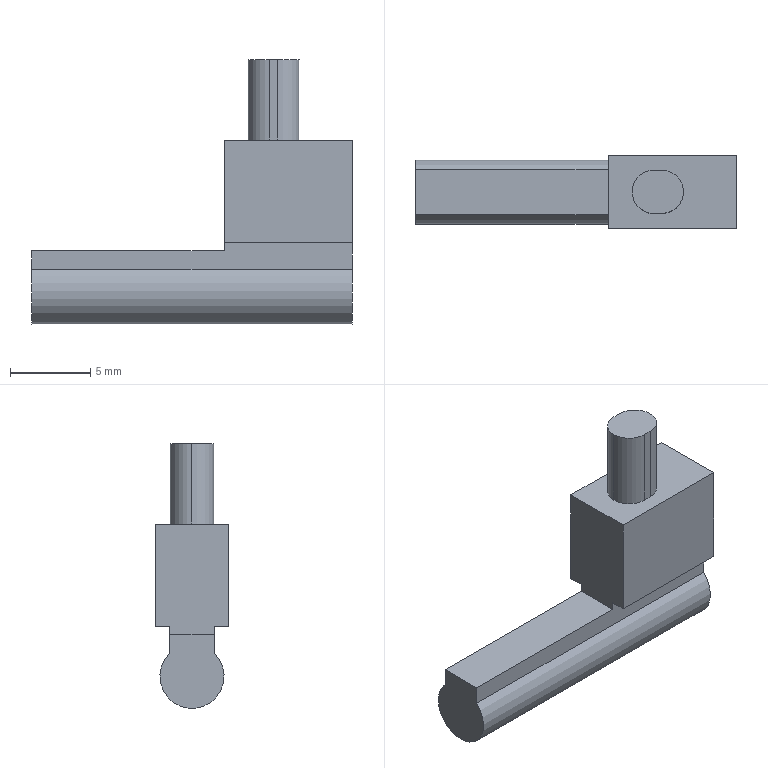Part | STEP file | 1105WWT8_1 | 1 solid | 18 faces | box 20 x 4.6 x 16.5 mm | volume 577.001 mm3 | plane 14 | cylinder 4 | commonest cylinder face diameters 2.7 x3 4 x1
STEP:
#1=CARTESIAN_POINT('',(34.85,8.,34.));
#2=VERTEX_POINT('',#1);
#3=CARTESIAN_POINT('',(33.5,9.35,34.));
#4=VERTEX_POINT('',#3);
#5=CARTESIAN_POINT('',(34.85,9.35,34.));
#6=DIRECTION('',(0.,0.,-1.));
#7=DIRECTION('',(-1.,0.,0.));
#8=AXIS2_PLACEMENT_3D('',#5,#6,#7);
#9=CIRCLE('',#8,1.35);
#10=EDGE_CURVE('',#2,#4,#9,.T.);
#11=ORIENTED_EDGE('',*,*,#10,.T.);
#12=CARTESIAN_POINT('',(33.5,9.35,29.));
#13=VERTEX_POINT('',#12);
#14=CARTESIAN_POINT('',(33.5,9.35,29.));
#15=DIRECTION('',(0.,0.,-1.));
#16=VECTOR('',#15,1000.);
#17=LINE('',#14,#16);
#18=EDGE_CURVE('',#4,#13,#17,.T.);
#19=ORIENTED_EDGE('',*,*,#18,.T.);
#20=CARTESIAN_POINT('',(34.85,8.,29.));
#21=VERTEX_POINT('',#20);
#22=CARTESIAN_POINT('',(34.85,9.35,29.));
#23=DIRECTION('',(0.,0.,-1.));
#24=DIRECTION('',(-1.,0.,0.));
#25=AXIS2_PLACEMENT_3D('',#22,#23,#24);
#26=CIRCLE('',#25,1.35);
#27=EDGE_CURVE('',#21,#13,#26,.T.);
#28=ORIENTED_EDGE('',*,*,#27,.F.);
#29=CARTESIAN_POINT('',(34.85,8.,29.));
#30=DIRECTION('',(0.,0.,1.));
#31=VECTOR('',#30,1000.);
#32=LINE('',#29,#31);
#33=EDGE_CURVE('',#21,#2,#32,.T.);
#34=ORIENTED_EDGE('',*,*,#33,.T.);
#35=EDGE_LOOP('',(#11,#19,#28,#34));
#36=FACE_OUTER_BOUND('',#35,.T.);
#37=CARTESIAN_POINT('',(34.85,9.35,29.));
#38=DIRECTION('',(0.,0.,-1.));
#39=DIRECTION('',(-1.,0.,0.));
#40=AXIS2_PLACEMENT_3D('',#37,#38,#39);
#41=CYLINDRICAL_SURFACE('',#40,1.35);
#42=ADVANCED_FACE('',(#36),#41,.T.);
#43=CARTESIAN_POINT('',(40.,7.95,20.928));
#44=VERTEX_POINT('',#43);
#45=CARTESIAN_POINT('',(20.,7.95,20.928));
#46=VERTEX_POINT('',#45);
#47=CARTESIAN_POINT('',(20.,7.95,20.928));
#48=DIRECTION('',(-1.,0.,0.));
#49=VECTOR('',#48,1000.);
#50=LINE('',#47,#49);
#51=EDGE_CURVE('',#44,#46,#50,.T.);
#52=ORIENTED_EDGE('',*,*,#51,.T.);
#53=CARTESIAN_POINT('',(20.,10.75,20.928));
#54=VERTEX_POINT('',#53);
#55=CARTESIAN_POINT('',(20.,9.35,19.5));
#56=DIRECTION('',(1.,0.,0.));
#57=DIRECTION('',(0.,0.,1.));
#58=AXIS2_PLACEMENT_3D('',#55,#56,#57);
#59=CIRCLE('',#58,2.);
#60=EDGE_CURVE('',#46,#54,#59,.T.);
#61=ORIENTED_EDGE('',*,*,#60,.T.);
#62=CARTESIAN_POINT('',(40.,10.75,20.928));
#63=VERTEX_POINT('',#62);
#64=CARTESIAN_POINT('',(20.,10.75,20.928));
#65=DIRECTION('',(1.,0.,0.));
#66=VECTOR('',#65,1000.);
#67=LINE('',#64,#66);
#68=EDGE_CURVE('',#54,#63,#67,.T.);
#69=ORIENTED_EDGE('',*,*,#68,.T.);
#70=CARTESIAN_POINT('',(40.,9.35,19.5));
#71=DIRECTION('',(-1.,0.,0.));
#72=DIRECTION('',(0.,0.,1.));
#73=AXIS2_PLACEMENT_3D('',#70,#71,#72);
#74=CIRCLE('',#73,2.);
#75=EDGE_CURVE('',#63,#44,#74,.T.);
#76=ORIENTED_EDGE('',*,*,#75,.T.);
#77=EDGE_LOOP('',(#52,#61,#69,#76));
#78=FACE_OUTER_BOUND('',#77,.T.);
#79=CARTESIAN_POINT('',(20.,9.35,19.5));
#80=DIRECTION('',(-1.,0.,0.));
#81=DIRECTION('',(0.,0.,1.));
#82=AXIS2_PLACEMENT_3D('',#79,#80,#81);
#83=CYLINDRICAL_SURFACE('',#82,2.);
#84=ADVANCED_FACE('',(#78),#83,.T.);
#85=CARTESIAN_POINT('',(20.,7.95,22.1));
#86=VERTEX_POINT('',#85);
#87=CARTESIAN_POINT('',(20.,7.95,19.5));
#88=DIRECTION('',(0.,0.,-1.));
#89=VECTOR('',#88,1000.);
#90=LINE('',#87,#89);
#91=EDGE_CURVE('',#86,#46,#90,.T.);
#92=ORIENTED_EDGE('',*,*,#91,.F.);
#93=CARTESIAN_POINT('',(20.,10.75,22.1));
#94=VERTEX_POINT('',#93);
#95=CARTESIAN_POINT('',(20.,9.35,22.1));
#96=DIRECTION('',(0.,-1.,0.));
#97=VECTOR('',#96,1000.);
#98=LINE('',#95,#97);
#99=EDGE_CURVE('',#94,#86,#98,.T.);
#100=ORIENTED_EDGE('',*,*,#99,.F.);
#101=CARTESIAN_POINT('',(20.,10.75,22.1));
#102=DIRECTION('',(0.,0.,1.));
#103=VECTOR('',#102,1000.);
#104=LINE('',#101,#103);
#105=EDGE_CURVE('',#54,#94,#104,.T.);
#106=ORIENTED_EDGE('',*,*,#105,.F.);
#107=ORIENTED_EDGE('',*,*,#60,.F.);
#108=EDGE_LOOP('',(#92,#100,#106,#107));
#109=FACE_OUTER_BOUND('',#108,.T.);
#110=CARTESIAN_POINT('',(20.,9.35,19.5));
#111=DIRECTION('',(1.,0.,0.));
#112=DIRECTION('',(0.,0.,-1.));
#113=AXIS2_PLACEMENT_3D('',#110,#111,#112);
#114=PLANE('',#113);
#115=ADVANCED_FACE('',(#109),#114,.F.);
#116=CARTESIAN_POINT('',(40.,7.95,22.6));
#117=VERTEX_POINT('',#116);
#118=CARTESIAN_POINT('',(32.,7.95,22.6));
#119=VERTEX_POINT('',#118);
#120=CARTESIAN_POINT('',(20.,7.95,22.6));
#121=DIRECTION('',(-1.,0.,0.));
#122=VECTOR('',#121,1000.);
#123=LINE('',#120,#122);
#124=EDGE_CURVE('',#117,#119,#123,.T.);
#125=ORIENTED_EDGE('',*,*,#124,.T.);
#126=CARTESIAN_POINT('',(32.,7.95,22.1));
#127=VERTEX_POINT('',#126);
#128=CARTESIAN_POINT('',(32.,7.95,19.5));
#129=DIRECTION('',(0.,0.,-1.));
#130=VECTOR('',#129,1000.);
#131=LINE('',#128,#130);
#132=EDGE_CURVE('',#119,#127,#131,.T.);
#133=ORIENTED_EDGE('',*,*,#132,.T.);
#134=CARTESIAN_POINT('',(20.,7.95,22.1));
#135=DIRECTION('',(-1.,0.,0.));
#136=VECTOR('',#135,1000.);
#137=LINE('',#134,#136);
#138=EDGE_CURVE('',#127,#86,#137,.T.);
#139=ORIENTED_EDGE('',*,*,#138,.T.);
#140=ORIENTED_EDGE('',*,*,#91,.T.);
#141=ORIENTED_EDGE('',*,*,#51,.F.);
#142=CARTESIAN_POINT('',(40.,7.95,20.928));
#143=DIRECTION('',(0.,0.,1.));
#144=VECTOR('',#143,1000.);
#145=LINE('',#142,#144);
#146=EDGE_CURVE('',#44,#117,#145,.T.);
#147=ORIENTED_EDGE('',*,*,#146,.T.);
#148=EDGE_LOOP('',(#125,#133,#139,#140,#141,#147));
#149=FACE_OUTER_BOUND('',#148,.T.);
#150=CARTESIAN_POINT('',(20.,7.95,20.928));
#151=DIRECTION('',(0.,-1.,0.));
#152=DIRECTION('',(0.,0.,-1.));
#153=AXIS2_PLACEMENT_3D('',#150,#151,#152);
#154=PLANE('',#153);
#155=ADVANCED_FACE('',(#149),#154,.T.);
#156=ORIENTED_EDGE('',*,*,#146,.F.);
#157=ORIENTED_EDGE('',*,*,#75,.F.);
#158=CARTESIAN_POINT('',(40.,10.75,22.6));
#159=VERTEX_POINT('',#158);
#160=CARTESIAN_POINT('',(40.,10.75,22.1));
#161=DIRECTION('',(0.,0.,-1.));
#162=VECTOR('',#161,1000.);
#163=LINE('',#160,#162);
#164=EDGE_CURVE('',#159,#63,#163,.T.);
#165=ORIENTED_EDGE('',*,*,#164,.F.);
#166=CARTESIAN_POINT('',(40.,11.65,22.6));
#167=VERTEX_POINT('',#166);
#168=CARTESIAN_POINT('',(40.,10.75,22.6));
#169=DIRECTION('',(0.,-1.,0.));
#170=VECTOR('',#169,1000.);
#171=LINE('',#168,#170);
#172=EDGE_CURVE('',#167,#159,#171,.T.);
#173=ORIENTED_EDGE('',*,*,#172,.F.);
#174=CARTESIAN_POINT('',(40.,11.65,29.));
#175=VERTEX_POINT('',#174);
#176=CARTESIAN_POINT('',(40.,11.65,19.5));
#177=DIRECTION('',(0.,0.,1.));
#178=VECTOR('',#177,1000.);
#179=LINE('',#176,#178);
#180=EDGE_CURVE('',#167,#175,#179,.T.);
#181=ORIENTED_EDGE('',*,*,#180,.T.);
#182=CARTESIAN_POINT('',(40.,7.05,29.));
#183=VERTEX_POINT('',#182);
#184=CARTESIAN_POINT('',(40.,9.35,29.));
#185=DIRECTION('',(0.,-1.,0.));
#186=VECTOR('',#185,1000.);
#187=LINE('',#184,#186);
#188=EDGE_CURVE('',#175,#183,#187,.T.);
#189=ORIENTED_EDGE('',*,*,#188,.T.);
#190=CARTESIAN_POINT('',(40.,7.05,22.6));
#191=VERTEX_POINT('',#190);
#192=CARTESIAN_POINT('',(40.,7.05,19.5));
#193=DIRECTION('',(0.,0.,-1.));
#194=VECTOR('',#193,1000.);
#195=LINE('',#192,#194);
#196=EDGE_CURVE('',#183,#191,#195,.T.);
#197=ORIENTED_EDGE('',*,*,#196,.T.);
#198=CARTESIAN_POINT('',(40.,9.35,22.6));
#199=DIRECTION('',(0.,1.,0.));
#200=VECTOR('',#199,1000.);
#201=LINE('',#198,#200);
#202=EDGE_CURVE('',#191,#117,#201,.T.);
#203=ORIENTED_EDGE('',*,*,#202,.T.);
#204=EDGE_LOOP('',(#156,#157,#165,#173,#181,#189,#197,#203));
#205=FACE_OUTER_BOUND('',#204,.T.);
#206=CARTESIAN_POINT('',(40.,9.35,19.5));
#207=DIRECTION('',(1.,0.,0.));
#208=DIRECTION('',(0.,0.,-1.));
#209=AXIS2_PLACEMENT_3D('',#206,#207,#208);
#210=PLANE('',#209);
#211=ADVANCED_FACE('',(#205),#210,.T.);
#212=ORIENTED_EDGE('',*,*,#99,.T.);
#213=ORIENTED_EDGE('',*,*,#138,.F.);
#214=CARTESIAN_POINT('',(32.,10.75,22.1));
#215=VERTEX_POINT('',#214);
#216=CARTESIAN_POINT('',(32.,7.95,22.1));
#217=DIRECTION('',(0.,1.,0.));
#218=VECTOR('',#217,1000.);
#219=LINE('',#216,#218);
#220=EDGE_CURVE('',#127,#215,#219,.T.);
#221=ORIENTED_EDGE('',*,*,#220,.T.);
#222=CARTESIAN_POINT('',(20.,10.75,22.1));
#223=DIRECTION('',(-1.,0.,0.));
#224=VECTOR('',#223,1000.);
#225=LINE('',#222,#224);
#226=EDGE_CURVE('',#215,#94,#225,.T.);
#227=ORIENTED_EDGE('',*,*,#226,.T.);
#228=EDGE_LOOP('',(#212,#213,#221,#227));
#229=FACE_OUTER_BOUND('',#228,.T.);
#230=CARTESIAN_POINT('',(20.,7.95,22.1));
#231=DIRECTION('',(0.,0.,1.));
#232=DIRECTION('',(1.,0.,0.));
#233=AXIS2_PLACEMENT_3D('',#230,#231,#232);
#234=PLANE('',#233);
#235=ADVANCED_FACE('',(#229),#234,.T.);
#236=ORIENTED_EDGE('',*,*,#202,.F.);
#237=CARTESIAN_POINT('',(32.,7.05,22.6));
#238=VERTEX_POINT('',#237);
#239=CARTESIAN_POINT('',(40.,7.05,22.6));
#240=DIRECTION('',(-1.,0.,0.));
#241=VECTOR('',#240,1000.);
#242=LINE('',#239,#241);
#243=EDGE_CURVE('',#191,#238,#242,.T.);
#244=ORIENTED_EDGE('',*,*,#243,.T.);
#245=CARTESIAN_POINT('',(32.,7.05,22.6));
#246=DIRECTION('',(0.,1.,0.));
#247=VECTOR('',#246,1000.);
#248=LINE('',#245,#247);
#249=EDGE_CURVE('',#238,#119,#248,.T.);
#250=ORIENTED_EDGE('',*,*,#249,.T.);
#251=ORIENTED_EDGE('',*,*,#124,.F.);
#252=EDGE_LOOP('',(#236,#244,#250,#251));
#253=FACE_OUTER_BOUND('',#252,.T.);
#254=CARTESIAN_POINT('',(40.,7.05,22.6));
#255=DIRECTION('',(0.,0.,-1.));
#256=DIRECTION('',(-1.,0.,0.));
#257=AXIS2_PLACEMENT_3D('',#254,#255,#256);
#258=PLANE('',#257);
#259=ADVANCED_FACE('',(#253),#258,.T.);
#260=ORIENTED_EDGE('',*,*,#196,.F.);
#261=CARTESIAN_POINT('',(32.,7.05,29.));
#262=VERTEX_POINT('',#261);
#263=CARTESIAN_POINT('',(40.,7.05,29.));
#264=DIRECTION('',(-1.,0.,0.));
#265=VECTOR('',#264,1000.);
#266=LINE('',#263,#265);
#267=EDGE_CURVE('',#183,#262,#266,.T.);
#268=ORIENTED_EDGE('',*,*,#267,.T.);
#269=CARTESIAN_POINT('',(32.,7.05,29.));
#270=DIRECTION('',(0.,0.,-1.));
#271=VECTOR('',#270,1000.);
#272=LINE('',#269,#271);
#273=EDGE_CURVE('',#262,#238,#272,.T.);
#274=ORIENTED_EDGE('',*,*,#273,.T.);
#275=ORIENTED_EDGE('',*,*,#243,.F.);
#276=EDGE_LOOP('',(#260,#268,#274,#275));
#277=FACE_OUTER_BOUND('',#276,.T.);
#278=CARTESIAN_POINT('',(40.,7.05,29.));
#279=DIRECTION('',(0.,-1.,0.));
#280=DIRECTION('',(0.,0.,-1.));
#281=AXIS2_PLACEMENT_3D('',#278,#279,#280);
#282=PLANE('',#281);
#283=ADVANCED_FACE('',(#277),#282,.T.);
#284=ORIENTED_EDGE('',*,*,#188,.F.);
#285=CARTESIAN_POINT('',(32.,11.65,29.));
#286=VERTEX_POINT('',#285);
#287=CARTESIAN_POINT('',(40.,11.65,29.));
#288=DIRECTION('',(-1.,0.,0.));
#289=VECTOR('',#288,1000.);
#290=LINE('',#287,#289);
#291=EDGE_CURVE('',#175,#286,#290,.T.);
#292=ORIENTED_EDGE('',*,*,#291,.T.);
#293=CARTESIAN_POINT('',(32.,11.65,29.));
#294=DIRECTION('',(0.,-1.,0.));
#295=VECTOR('',#294,1000.);
#296=LINE('',#293,#295);
#297=EDGE_CURVE('',#286,#262,#296,.T.);
#298=ORIENTED_EDGE('',*,*,#297,.T.);
#299=ORIENTED_EDGE('',*,*,#267,.F.);
#300=EDGE_LOOP('',(#284,#292,#298,#299));
#301=FACE_OUTER_BOUND('',#300,.T.);
#302=CARTESIAN_POINT('',(35.35,10.7,29.));
#303=VERTEX_POINT('',#302);
#304=CARTESIAN_POINT('',(35.35,8.,29.));
#305=VERTEX_POINT('',#304);
#306=CARTESIAN_POINT('',(35.35,9.35,29.));
#307=DIRECTION('',(0.,0.,-1.));
#308=DIRECTION('',(-1.,0.,0.));
#309=AXIS2_PLACEMENT_3D('',#306,#307,#308);
#310=CIRCLE('',#309,1.35);
#311=EDGE_CURVE('',#303,#305,#310,.T.);
#312=ORIENTED_EDGE('',*,*,#311,.T.);
#313=CARTESIAN_POINT('',(35.35,8.,29.));
#314=DIRECTION('',(1.,0.,0.));
#315=VECTOR('',#314,1000.);
#316=LINE('',#313,#315);
#317=EDGE_CURVE('',#21,#305,#316,.T.);
#318=ORIENTED_EDGE('',*,*,#317,.F.);
#319=ORIENTED_EDGE('',*,*,#27,.T.);
#320=CARTESIAN_POINT('',(34.85,10.7,29.));
#321=VERTEX_POINT('',#320);
#322=CARTESIAN_POINT('',(34.85,9.35,29.));
#323=DIRECTION('',(0.,0.,-1.));
#324=DIRECTION('',(-1.,0.,0.));
#325=AXIS2_PLACEMENT_3D('',#322,#323,#324);
#326=CIRCLE('',#325,1.35);
#327=EDGE_CURVE('',#13,#321,#326,.T.);
#328=ORIENTED_EDGE('',*,*,#327,.T.);
#329=CARTESIAN_POINT('',(34.85,10.7,29.));
#330=DIRECTION('',(-1.,0.,0.));
#331=VECTOR('',#330,1000.);
#332=LINE('',#329,#331);
#333=EDGE_CURVE('',#303,#321,#332,.T.);
#334=ORIENTED_EDGE('',*,*,#333,.F.);
#335=EDGE_LOOP('',(#312,#318,#319,#328,#334));
#336=FACE_BOUND('',#335,.T.);
#337=CARTESIAN_POINT('',(40.,11.65,29.));
#338=DIRECTION('',(0.,0.,1.));
#339=DIRECTION('',(1.,0.,0.));
#340=AXIS2_PLACEMENT_3D('',#337,#338,#339);
#341=PLANE('',#340);
#342=ADVANCED_FACE('',(#301,#336),#341,.T.);
#343=ORIENTED_EDGE('',*,*,#180,.F.);
#344=CARTESIAN_POINT('',(32.,11.65,22.6));
#345=VERTEX_POINT('',#344);
#346=CARTESIAN_POINT('',(40.,11.65,22.6));
#347=DIRECTION('',(-1.,0.,0.));
#348=VECTOR('',#347,1000.);
#349=LINE('',#346,#348);
#350=EDGE_CURVE('',#167,#345,#349,.T.);
#351=ORIENTED_EDGE('',*,*,#350,.T.);
#352=CARTESIAN_POINT('',(32.,11.65,22.6));
#353=DIRECTION('',(0.,0.,1.));
#354=VECTOR('',#353,1000.);
#355=LINE('',#352,#354);
#356=EDGE_CURVE('',#345,#286,#355,.T.);
#357=ORIENTED_EDGE('',*,*,#356,.T.);
#358=ORIENTED_EDGE('',*,*,#291,.F.);
#359=EDGE_LOOP('',(#343,#351,#357,#358));
#360=FACE_OUTER_BOUND('',#359,.T.);
#361=CARTESIAN_POINT('',(40.,11.65,22.6));
#362=DIRECTION('',(0.,1.,0.));
#363=DIRECTION('',(0.,0.,1.));
#364=AXIS2_PLACEMENT_3D('',#361,#362,#363);
#365=PLANE('',#364);
#366=ADVANCED_FACE('',(#360),#365,.T.);
#367=CARTESIAN_POINT('',(32.,10.75,22.6));
#368=VERTEX_POINT('',#367);
#369=CARTESIAN_POINT('',(20.,10.75,22.6));
#370=DIRECTION('',(1.,0.,0.));
#371=VECTOR('',#370,1000.);
#372=LINE('',#369,#371);
#373=EDGE_CURVE('',#368,#159,#372,.T.);
#374=ORIENTED_EDGE('',*,*,#373,.T.);
#375=ORIENTED_EDGE('',*,*,#164,.T.);
#376=ORIENTED_EDGE('',*,*,#68,.F.);
#377=ORIENTED_EDGE('',*,*,#105,.T.);
#378=ORIENTED_EDGE('',*,*,#226,.F.);
#379=CARTESIAN_POINT('',(32.,10.75,22.1));
#380=DIRECTION('',(0.,0.,1.));
#381=VECTOR('',#380,1000.);
#382=LINE('',#379,#381);
#383=EDGE_CURVE('',#215,#368,#382,.T.);
#384=ORIENTED_EDGE('',*,*,#383,.T.);
#385=EDGE_LOOP('',(#374,#375,#376,#377,#378,#384));
#386=FACE_OUTER_BOUND('',#385,.T.);
#387=CARTESIAN_POINT('',(20.,10.75,22.1));
#388=DIRECTION('',(0.,1.,0.));
#389=DIRECTION('',(0.,0.,1.));
#390=AXIS2_PLACEMENT_3D('',#387,#388,#389);
#391=PLANE('',#390);
#392=ADVANCED_FACE('',(#386),#391,.T.);
#393=ORIENTED_EDGE('',*,*,#132,.F.);
#394=ORIENTED_EDGE('',*,*,#249,.F.);
#395=ORIENTED_EDGE('',*,*,#273,.F.);
#396=ORIENTED_EDGE('',*,*,#297,.F.);
#397=ORIENTED_EDGE('',*,*,#356,.F.);
#398=CARTESIAN_POINT('',(32.,9.35,22.6));
#399=DIRECTION('',(0.,1.,0.));
#400=VECTOR('',#399,1000.);
#401=LINE('',#398,#400);
#402=EDGE_CURVE('',#368,#345,#401,.T.);
#403=ORIENTED_EDGE('',*,*,#402,.F.);
#404=ORIENTED_EDGE('',*,*,#383,.F.);
#405=ORIENTED_EDGE('',*,*,#220,.F.);
#406=EDGE_LOOP('',(#393,#394,#395,#396,#397,#403,#404,#405));
#407=FACE_OUTER_BOUND('',#406,.T.);
#408=CARTESIAN_POINT('',(32.,9.35,19.5));
#409=DIRECTION('',(1.,0.,0.));
#410=DIRECTION('',(0.,0.,-1.));
#411=AXIS2_PLACEMENT_3D('',#408,#409,#410);
#412=PLANE('',#411);
#413=ADVANCED_FACE('',(#407),#412,.F.);
#414=ORIENTED_EDGE('',*,*,#311,.F.);
#415=CARTESIAN_POINT('',(35.35,10.7,34.));
#416=VERTEX_POINT('',#415);
#417=CARTESIAN_POINT('',(35.35,10.7,29.));
#418=DIRECTION('',(0.,0.,1.));
#419=VECTOR('',#418,1000.);
#420=LINE('',#417,#419);
#421=EDGE_CURVE('',#303,#416,#420,.T.);
#422=ORIENTED_EDGE('',*,*,#421,.T.);
#423=CARTESIAN_POINT('',(35.35,8.,34.));
#424=VERTEX_POINT('',#423);
#425=CARTESIAN_POINT('',(35.35,9.35,34.));
#426=DIRECTION('',(0.,0.,-1.));
#427=DIRECTION('',(-1.,0.,0.));
#428=AXIS2_PLACEMENT_3D('',#425,#426,#427);
#429=CIRCLE('',#428,1.35);
#430=EDGE_CURVE('',#416,#424,#429,.T.);
#431=ORIENTED_EDGE('',*,*,#430,.T.);
#432=CARTESIAN_POINT('',(35.35,8.,29.));
#433=DIRECTION('',(0.,0.,-1.));
#434=VECTOR('',#433,1000.);
#435=LINE('',#432,#434);
#436=EDGE_CURVE('',#424,#305,#435,.T.);
#437=ORIENTED_EDGE('',*,*,#436,.T.);
#438=EDGE_LOOP('',(#414,#422,#431,#437));
#439=FACE_OUTER_BOUND('',#438,.T.);
#440=CARTESIAN_POINT('',(35.35,9.35,29.));
#441=DIRECTION('',(0.,0.,-1.));
#442=DIRECTION('',(-1.,0.,0.));
#443=AXIS2_PLACEMENT_3D('',#440,#441,#442);
#444=CYLINDRICAL_SURFACE('',#443,1.35);
#445=ADVANCED_FACE('',(#439),#444,.T.);
#446=ORIENTED_EDGE('',*,*,#18,.F.);
#447=CARTESIAN_POINT('',(34.85,10.7,34.));
#448=VERTEX_POINT('',#447);
#449=CARTESIAN_POINT('',(34.85,9.35,34.));
#450=DIRECTION('',(0.,0.,-1.));
#451=DIRECTION('',(-1.,0.,0.));
#452=AXIS2_PLACEMENT_3D('',#449,#450,#451);
#453=CIRCLE('',#452,1.35);
#454=EDGE_CURVE('',#4,#448,#453,.T.);
#455=ORIENTED_EDGE('',*,*,#454,.T.);
#456=CARTESIAN_POINT('',(34.85,10.7,29.));
#457=DIRECTION('',(0.,0.,-1.));
#458=VECTOR('',#457,1000.);
#459=LINE('',#456,#458);
#460=EDGE_CURVE('',#448,#321,#459,.T.);
#461=ORIENTED_EDGE('',*,*,#460,.T.);
#462=ORIENTED_EDGE('',*,*,#327,.F.);
#463=EDGE_LOOP('',(#446,#455,#461,#462));
#464=FACE_OUTER_BOUND('',#463,.T.);
#465=CARTESIAN_POINT('',(34.85,9.35,29.));
#466=DIRECTION('',(0.,0.,-1.));
#467=DIRECTION('',(-1.,0.,0.));
#468=AXIS2_PLACEMENT_3D('',#465,#466,#467);
#469=CYLINDRICAL_SURFACE('',#468,1.35);
#470=ADVANCED_FACE('',(#464),#469,.T.);
#471=ORIENTED_EDGE('',*,*,#172,.T.);
#472=ORIENTED_EDGE('',*,*,#373,.F.);
#473=ORIENTED_EDGE('',*,*,#402,.T.);
#474=ORIENTED_EDGE('',*,*,#350,.F.);
#475=EDGE_LOOP('',(#471,#472,#473,#474));
#476=FACE_OUTER_BOUND('',#475,.T.);
#477=CARTESIAN_POINT('',(40.,10.75,22.6));
#478=DIRECTION('',(0.,0.,-1.));
#479=DIRECTION('',(-1.,0.,0.));
#480=AXIS2_PLACEMENT_3D('',#477,#478,#479);
#481=PLANE('',#480);
#482=ADVANCED_FACE('',(#476),#481,.T.);
#483=ORIENTED_EDGE('',*,*,#333,.T.);
#484=ORIENTED_EDGE('',*,*,#460,.F.);
#485=CARTESIAN_POINT('',(34.85,10.7,34.));
#486=DIRECTION('',(1.,0.,0.));
#487=VECTOR('',#486,1000.);
#488=LINE('',#485,#487);
#489=EDGE_CURVE('',#448,#416,#488,.T.);
#490=ORIENTED_EDGE('',*,*,#489,.T.);
#491=ORIENTED_EDGE('',*,*,#421,.F.);
#492=EDGE_LOOP('',(#483,#484,#490,#491));
#493=FACE_OUTER_BOUND('',#492,.T.);
#494=CARTESIAN_POINT('',(34.85,10.7,29.));
#495=DIRECTION('',(0.,1.,0.));
#496=DIRECTION('',(0.,0.,1.));
#497=AXIS2_PLACEMENT_3D('',#494,#495,#496);
#498=PLANE('',#497);
#499=ADVANCED_FACE('',(#493),#498,.T.);
#500=ORIENTED_EDGE('',*,*,#317,.T.);
#501=ORIENTED_EDGE('',*,*,#436,.F.);
#502=CARTESIAN_POINT('',(35.35,8.,34.));
#503=DIRECTION('',(-1.,0.,0.));
#504=VECTOR('',#503,1000.);
#505=LINE('',#502,#504);
#506=EDGE_CURVE('',#424,#2,#505,.T.);
#507=ORIENTED_EDGE('',*,*,#506,.T.);
#508=ORIENTED_EDGE('',*,*,#33,.F.);
#509=EDGE_LOOP('',(#500,#501,#507,#508));
#510=FACE_OUTER_BOUND('',#509,.T.);
#511=CARTESIAN_POINT('',(35.35,8.,29.));
#512=DIRECTION('',(0.,-1.,0.));
#513=DIRECTION('',(0.,0.,-1.));
#514=AXIS2_PLACEMENT_3D('',#511,#512,#513);
#515=PLANE('',#514);
#516=ADVANCED_FACE('',(#510),#515,.T.);
#517=ORIENTED_EDGE('',*,*,#430,.F.);
#518=ORIENTED_EDGE('',*,*,#489,.F.);
#519=ORIENTED_EDGE('',*,*,#454,.F.);
#520=ORIENTED_EDGE('',*,*,#10,.F.);
#521=ORIENTED_EDGE('',*,*,#506,.F.);
#522=EDGE_LOOP('',(#517,#518,#519,#520,#521));
#523=FACE_OUTER_BOUND('',#522,.T.);
#524=CARTESIAN_POINT('',(20.,9.35,34.));
#525=DIRECTION('',(0.,0.,1.));
#526=DIRECTION('',(1.,0.,0.));
#527=AXIS2_PLACEMENT_3D('',#524,#525,#526);
#528=PLANE('',#527);
#529=ADVANCED_FACE('',(#523),#528,.T.);
#530=CLOSED_SHELL('',(#42,#84,#115,#155,#211,#235,#259,#283,#342,#366,#392,#413,#445,#470,#482,#499,#516,#529));
#531=MANIFOLD_SOLID_BREP('',#530);
#532=CARTESIAN_POINT('',(0.,0.,0.));
#533=DIRECTION('',(0.,0.,1.));
#534=DIRECTION('',(1.,0.,0.));
#535=AXIS2_PLACEMENT_3D('',#532,#533,#534);
#536=(LENGTH_UNIT()NAMED_UNIT(*)SI_UNIT(.MILLI.,.METRE.));
#537=UNCERTAINTY_MEASURE_WITH_UNIT(LENGTH_MEASURE(0.00001),#536,'','');
#538=(NAMED_UNIT(*)PLANE_ANGLE_UNIT()SI_UNIT($,.RADIAN.));
#539=(NAMED_UNIT(*)SI_UNIT($,.STERADIAN.)SOLID_ANGLE_UNIT());
#540=(GEOMETRIC_REPRESENTATION_CONTEXT(3)GLOBAL_UNCERTAINTY_ASSIGNED_CONTEXT((#537))GLOBAL_UNIT_ASSIGNED_CONTEXT((#536,#538,#539))REPRESENTATION_CONTEXT('',''));
#541=ADVANCED_BREP_SHAPE_REPRESENTATION('',(#531,#535),#540);